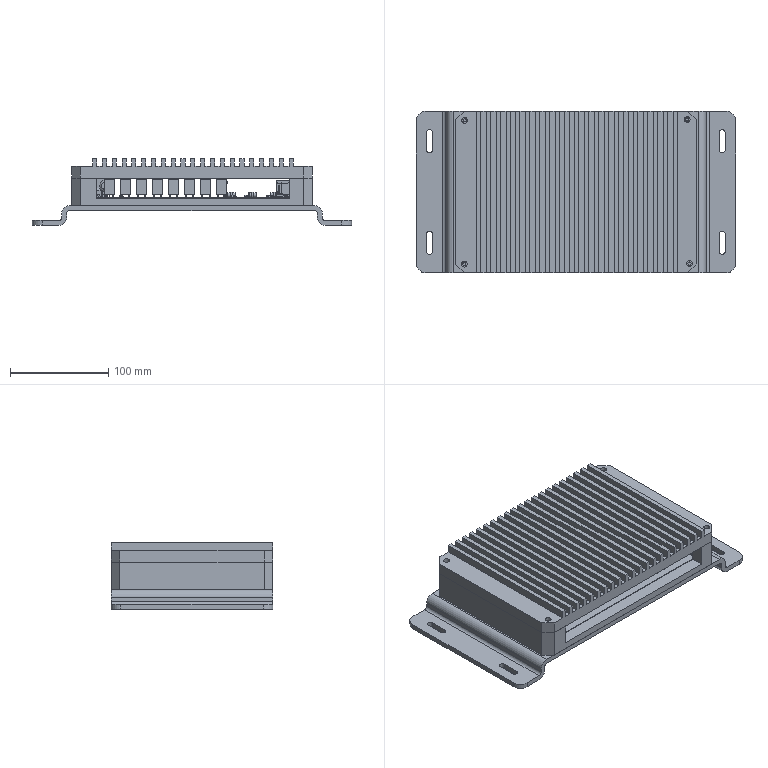Part | NX | features BREP 54 | 106 solids | 8556 faces | volume 1246093 mm3 | plane 4986 | spline 2019 | cylinder 1447 | torus 66 | cone 26 | sphere 12 | commonest cylinder face diameters 0.305 x732 1.2 x200 1 x100 0.681 x54 0.157 x36 0.674 x36